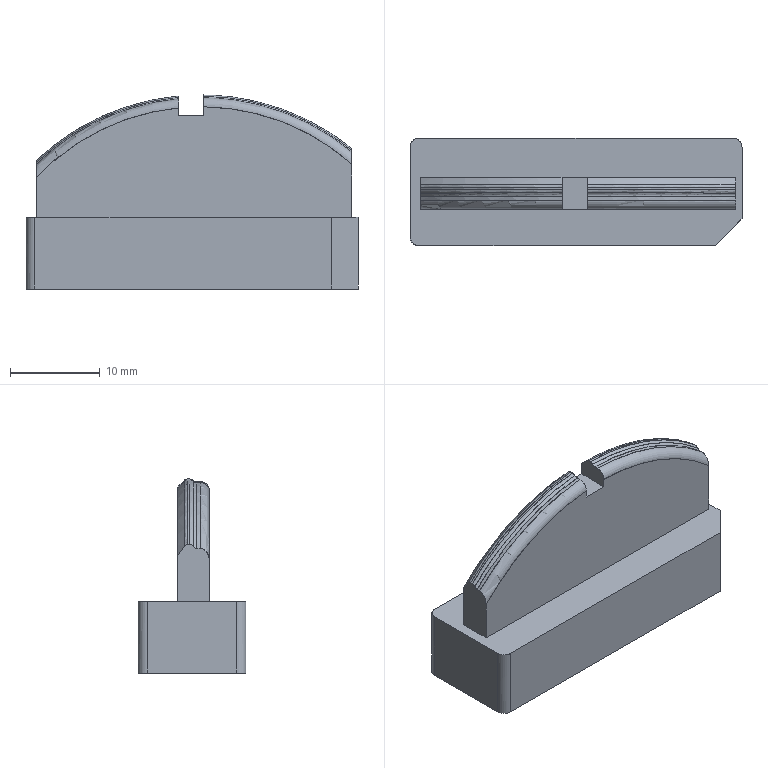NC program | PowerMill | posted with a generic post | part box 37 x 12 x 21.629 mm
Lines 1 to 1018 of 105205:
%
O0001
N104 ( POWERMILL CB  : 2026004.0)
N105 ( POST VER      : 2026.0.0.5161)
N106 ( OPTION FILE   : FANUC)
N107 ( OUTPUT WORKPLANE : WORLD)
N108 (  )
N109 ( TOOL LIST )
N110 (---------------------------------------)
N111 ( NO. | ID        | DIA.| TIP RAD|LENGTH)
N112 (---------------------------------------)
N113 (    1|D10C_1_1_1 |10.0 |  0.0   |77.08 )
N114 (    2|D4C_1_1    | 4.0 |  0.0   | 68.8 )
N115 (   28|D2C_1_1    | 2.0 |  0.0   |57.56 )
N116 (    3|D10_1_1_1  |10.0 |  0.0   | 76.8 )
N117 (    4|R1_1_1     | 2.0 |  1.0   |65.24 )
N118 (   12|D2_1_1     | 2.0 |  0.0   |57.68 )
N119 (    6|R0.5_1_1   | 1.0 |  0.5   | 63.2 )
N120 (   13|TEXT_D4_1_1| 4.0 |  0.3   |68.88 )
N121 (---------------------------------------)
N122 (  )
N123 ( NUMBER OF TOOLPATHS: 12.0 )
N124 ( ESTIMATED PROGRAM DURATION: 0 HOURS 8 MIN 47 SEC)
N125 (  )
N126 G00 G21 G80 G40 G17
N127 G90
N128 G54
N129 G53 Z0.0
N130 (---------------)
N131 ( START TOOLPATH : 精公开粗01-扫面平行-D10C )
N132 (---------------)
N133 ( TOOL NO.    :1 )
N134 ( TOOL TYPE   : ENDMILL)
N135 ( TOOL ID     : D10C_1_1_1)
N136 ( TOOL DIA    : 10.0 LENGTH 77.08)
N137 T1
N138 M6
N139 S8000 M03
N140 G00 G90 X0.0 Y0.0
N141 G43 Z10.2 H1
N142
N143 G05 P10000 R4
N144 X26.28 Y8.78
N145 Z1.129
N146 G01 Z-0.071 F6000.0
N147 X21.28 F10000.0
N148 X-21.28
N149 Y2.9267
N150 X21.28
N151 Y-2.9267
N152 X-21.28
N153 Y-8.78
N154 X21.28
N155 X26.28
N156 G00 Z10.2
N157 G05 P0
N158 (---------------)
N159 ( END TOOLPATH : 精公开粗01-扫面平行-D10C )
N160 (---------------)
N161 ( START TOOLPATH : 精公开粗01-外形偏置-D10C )
N162 (---------------)
N163 G00 X0.242 Y-0.1675 Z9.879
N164 G05 P10000 R4
N165 X-3.7058 Y14.649
N166 Z0.6814
N167 G01 Z-0.5186 F6000.0
N168 Y14.1215 F10000.0
N169 G03 X1.0417 Y9.374 I4.7475 J0.0
N170 G01 X24.573
N171 G02 X25.573 Y8.374 I0.0 J-1.0
N172 G01 Y-8.709
N173 G02 X24.573 Y-9.709 I-1.0 J0.0
N174 G01 X-24.089
N175 G02 X-25.089 Y-8.709 I0.0 J1.0
N176 G01 Y8.374
N177 G02 X-24.089 Y9.374 I1.0 J0.0
N178 G01 X1.0417
N179 X1.2088 Y6.3133
N180 X1.4021 Y6.3238
N181 X2.949 Y6.2597
N182 X3.7224 Y6.2023
N183 X5.3688 Y6.0199
N184 X6.0427 Y5.8933
N185 X6.8161 Y5.6829
N186 X7.5896 Y5.3718
N187 X7.8472 Y5.2465
N188 X8.363 Y4.9346
N189 X8.9527 Y4.4731
N190 X9.6513 Y3.6996
N191 X9.9098 Y3.3388
N192 X10.1534 Y2.9262
N193 X10.4864 Y2.1528
N194 X10.6833 Y1.3714
N195 X10.7117 Y1.0849
N196 X16.2576 Y1.3418
N197 X16.2439 Y1.6377
N198 G02 X17.3399 Y3.2854 I1.6702 J0.0774
N199 G01 X17.6988 Y3.4167
N200 G02 X19.945 Y1.8531 I0.5742 J-1.5703
N201 G01 X19.9612 Y-2.1531
N202 G02 X17.0031 Y-3.5452 I-1.8032 J-0.0073
N203 G01 X16.7549 Y-3.3382
N204 G02 X16.1376 Y-1.8427 I1.1128 J1.3345
N205 G01 X16.2447 Y-0.6921
N206 X16.2894 Y0.0777
N207 X16.2805 Y0.8487
N208 X16.2576 Y1.3418
N209 X10.7117 Y1.0849
N210 X10.7593 Y0.6059
N211 X10.7454 Y-0.1675
N212 X10.6264 Y-0.9409
N213 X10.3838 Y-1.7144
N214 X9.9952 Y-2.4878
N215 X9.4263 Y-3.2612
N216 X9.1364 Y-3.5758
N217 X8.6195 Y-4.0346
N218 X8.363 Y-4.2201
N219 X7.5896 Y-4.654
N220 X6.8161 Y-4.966
N221 X6.1624 Y-5.1488
N222 X6.0948 Y-5.173
N223 X6.0314 Y-5.2067
N224 X5.4336 Y-5.5815
N225 X4.4958 Y-6.0392
N226 X3.7224 Y-6.2668
N227 X3.2355 Y-6.3549
N228 X2.949 Y-6.3912
N229 X1.4021 Y-6.5336
N230 X0.6287 Y-6.4969
N231 X-0.1003 Y-6.3549
N232 X-0.9181 Y-6.0598
N233 X-1.7384 Y-5.5794
N234 X-1.8347 Y-5.536
N235 X-1.9379 Y-5.5137
N236 X-2.465 Y-5.4572
N237 X-4.0118 Y-5.1831
N238 X-4.7853 Y-4.9732
N239 X-5.5587 Y-4.6686
N240 X-6.3321 Y-4.2406
N241 X-6.6232 Y-4.0346
N242 X-7.1056 Y-3.6105
N243 X-7.449 Y-3.2612
N244 X-8.0238 Y-2.4878
N245 X-8.4121 Y-1.7144
N246 X-8.6539 Y-0.9409
N247 X-8.6938 Y-0.6802
N248 X-14.3983 Y-1.0073
N249 X-14.3455 Y-1.9276
N250 G02 X-16.8483 Y-3.977 I-1.9967 J-0.1145
N251 G01 X-17.7043 Y-3.7531
N252 G02 X-19.1982 Y-1.8182 I0.5061 J1.9349
N253 G01 Y1.4832
N254 G02 X-17.6684 Y3.4271 I2.0 J0.0
N255 G01 X-17.0235 Y3.5831
N256 G02 X-14.5566 Y1.7537 I0.4702 J-1.9439
N257 G01 X-14.3983 Y-1.0073
N258 X-8.6938 Y-0.6802
N259 X-8.7721 Y-0.1675
N260 X-8.7879 Y0.6059
N261 X-8.7101 Y1.3794
N262 X-8.5124 Y2.1528
N263 X-8.1804 Y2.9262
N264 X-7.879 Y3.4159
N265 X-7.6758 Y3.6996
N266 X-7.1056 Y4.3308
N267 X-6.3321 Y4.9568
N268 X-5.8498 Y5.2465
N269 X-5.5587 Y5.3869
N270 X-4.7853 Y5.69
N271 X-4.0118 Y5.8981
N272 X-3.3512 Y6.0199
N273 X-1.6916 Y6.2012
N274 X-0.9181 Y6.1653
N275 X-0.4581 Y6.0835
N276 X-0.3402 Y6.0767
N277 X-0.224 Y6.0977
N278 X-0.1447 Y6.122
N279 X0.6287 Y6.2816
N280 X1.2088 Y6.3133
N281 X1.0417 Y9.374
N282 G00 Z3.2838
N283 G01 X-3.7058 Y14.649
N284 G00 Z0.2838
N285 G01 Z-0.9162 F6000.0
N286 Y14.1215 F10000.0
N287 G03 X1.0417 Y9.374 I4.7475 J0.0
N288 G01 X24.573
N289 G02 X25.573 Y8.374 I0.0 J-1.0
N290 G01 Y-0.2376
N291 X19.8931 Y-0.1574
N292 X19.8544 Y-2.8993
N293 G02 X18.8442 Y-3.6348 I-0.7809 J0.011
N294 G01 X18.4957 Y-3.5278
N295 G02 X17.9956 Y-2.7453 I0.2105 J0.6856
N296 G01 X18.2091 Y-1.18
N297 G03 X18.2459 Y1.5707 I-11.186 J1.5254
N298 G01 X18.1442 Y2.5018
N299 G02 X18.6817 Y3.1923 I0.6248 J0.0682
N300 G01 X19.1656 Y3.2602
N301 G02 X19.9318 Y2.5844 I0.0935 J-0.6663
N302 G01 X19.8931 Y-0.1574
N303 X25.573 Y-0.2376
N304 Y-8.709
N305 G02 X24.573 Y-9.709 I-1.0 J0.0
N306 G01 X-24.089
N307 G02 X-25.089 Y-8.709 I0.0 J1.0
N308 G01 Y8.374
N309 G02 X-24.089 Y9.374 I1.0 J0.0
N310 G01 X0.9629
N311 X1.1121 Y6.7052
N312 X1.4021 Y6.7215
N313 X2.949 Y6.6563
N314 X3.7224 Y6.5978
N315 X5.2693 Y6.4317
N316 X7.5896 Y6.0268
N317 X8.363 Y5.8328
N318 X9.1364 Y5.576
N319 X9.804 Y5.2465
N320 X10.6833 Y4.6509
N321 X10.8898 Y4.4731
N322 X11.5828 Y3.6996
N323 X12.0614 Y2.9262
N324 X12.2301 Y2.573
N325 X12.3936 Y2.1528
N326 X12.5912 Y1.3794
N327 X12.6666 Y0.6059
N328 X12.6539 Y-0.1675
N329 X12.5353 Y-0.9409
N330 X12.2911 Y-1.7144
N331 X11.9079 Y-2.4878
N332 X11.3639 Y-3.2612
N333 X10.6833 Y-3.9336
N334 X9.8625 Y-4.4919
N335 X9.8122 Y-4.5311
N336 X9.7673 Y-4.5763
N337 X9.7224 Y-4.6276
N338 X9.1364 Y-5.1826
N339 X8.5886 Y-5.5815
N340 X7.5896 Y-6.1042
N341 X6.956 Y-6.3549
N342 X6.0427 Y-6.6013
N343 X5.2693 Y-6.7489
N344 X4.4958 Y-6.8496
N345 X2.949 Y-6.9772
N346 X1.4021 Y-7.0238
N347 X0.6287 Y-6.9871
N348 X-0.2047 Y-6.8115
N349 X-0.2986 Y-6.8008
N350 X-0.3928 Y-6.808
N351 X-0.9181 Y-6.8986
N352 X-1.6916 Y-6.9275
N353 X-2.465 Y-6.8575
N354 X-3.2384 Y-6.7562
N355 X-4.0118 Y-6.6086
N356 X-4.7853 Y-6.4026
N357 X-5.5587 Y-6.1159
N358 X-6.3321 Y-5.741
N359 X-6.6106 Y-5.5815
N360 X-7.1056 Y-5.2246
N361 X-7.5738 Y-4.8081
N362 X-7.8388 Y-4.5227
N363 X-7.8812 Y-4.4822
N364 X-7.9281 Y-4.4468
N365 X-8.5473 Y-4.0346
N366 X-9.3538 Y-3.2612
N367 X-9.8919 Y-2.4878
N368 X-10.2739 Y-1.7144
N369 X-10.5168 Y-0.9409
N370 X-10.635 Y-0.1675
N371 Y-0.1658
N372 X-16.2712 Y-0.4157
N373 X-16.2674 Y-0.5009
N374 X-16.1342 Y-2.2825
N375 G02 X-17.6603 Y-4.0077 I-1.6027 J-0.1199
N376 G02 X-19.3438 Y-2.4356 I-0.0766 J1.6053
N377 G01 X-19.4362 Y2.0303
N378 G02 X-16.8686 Y3.1779 I1.5262 J0.0316
N379 G01 X-16.7304 Y3.0489
N380 G02 X-16.2734 Y1.9733 I-0.9816 J-1.0519
N381 G01 X-16.2977 Y0.1812
N382 X-16.2712 Y-0.4157
N383 X-10.635 Y-0.1658
N384 X-10.6489 Y0.6059
N385 X-10.573 Y1.3794
N386 X-10.3765 Y2.1528
N387 X-10.1993 Y2.6067
N388 X-10.044 Y2.9262
N389 X-9.569 Y3.6996
N390 X-9.4258 Y3.89
N391 X-8.8796 Y4.4731
N392 X-8.6524 Y4.6669
N393 X-7.879 Y5.1956
N394 X-7.1056 Y5.5891
N395 X-6.3321 Y5.8469
N396 X-5.5587 Y6.0303
N397 X-4.0118 Y6.322
N398 X-2.465 Y6.5244
N399 X-1.6916 Y6.5964
N400 X-0.9181 Y6.5595
N401 X-0.4624 Y6.4781
N402 X-0.3447 Y6.4711
N403 X-0.2286 Y6.492
N404 X-0.1447 Y6.5176
N405 X0.6287 Y6.6782
N406 X1.1121 Y6.7052
N407 X0.9629 Y9.374
N408 X1.0417
N409 G00 Z2.8861
N410 G01 X-3.7058 Y14.649
N411 G00 Z-0.1139
N412 G01 Z-1.3139 F6000.0
N413 Y14.1215 F10000.0
N414 G03 X1.0417 Y9.374 I4.7475 J0.0
N415 G01 X2.9512
N416 X2.949 Y6.8729
N417 X4.4958 Y6.8716
N418 X5.4708 Y6.7933
N419 X7.5896 Y6.414
N420 X9.1364 Y6.0561
N421 X9.9098 Y5.8404
N422 X10.6833 Y5.5459
N423 X11.4567 Y5.1307
N424 X12.2301 Y4.5478
N425 X13.0107 Y3.6996
N426 X13.4819 Y2.9262
N427 X13.777 Y2.2408
N428 X14.0066 Y1.3794
N429 X14.0825 Y0.6059
N430 X14.0678 Y-0.1675
N431 X13.95 Y-0.9409
N432 X13.777 Y-1.5309
N433 X13.3301 Y-2.4878
N434 X13.0035 Y-2.9907
N435 X12.7928 Y-3.2612
N436 X12.2301 Y-3.8366
N437 X12.014 Y-4.0144
N438 X11.9644 Y-4.0612
N439 X11.9216 Y-4.1143
N440 X11.4567 Y-4.6934
N441 X10.6833 Y-5.3869
N442 X9.9098 Y-5.9011
N443 X9.1364 Y-6.2674
N444 X8.363 Y-6.5411
N445 X7.5896 Y-6.7396
N446 X6.8161 Y-6.894
N447 X5.2693 Y-7.0717
N448 X4.2297 Y-7.1283
N449 X1.4021 Y-7.1856
N450 X0.6287 Y-7.1515
N451 X-0.0851 Y-7.0102
N452 X-0.1785 Y-7.0007
N453 X-0.2721 Y-7.0089
N454 X-0.9181 Y-7.1269
N455 X-1.6916 Y-7.1557
N456 X-3.2384 Y-7.0743
N457 X-4.7853 Y-6.9012
N458 X-5.5587 Y-6.7449
N459 X-6.3321 Y-6.5514
N460 X-6.9147 Y-6.3549
N461 X-7.879 Y-5.9193
N462 X-8.6524 Y-5.3943
N463 X-9.334 Y-4.8081
N464 X-9.7128 Y-4.3808
N465 X-9.8966 Y-4.1287
N466 X-9.9372 Y-4.08
N467 X-9.9835 Y-4.0368
N468 X-10.1993 Y-3.8598
N469 X-10.7912 Y-3.2612
N470 X-10.9727 Y-3.0292
N471 X-11.3287 Y-2.4878
N472 X-11.7125 Y-1.7144
N473 X-11.8563 Y-1.2605
N474 X-17.1845 Y-2.3028
N475 X-17.1233 Y-2.6155
N476 G02 X-17.5543 Y-3.7187 I-1.0844 J-0.2122
N477 G01 X-17.7752 Y-3.8806
N478 G02 X-19.6195 Y-2.9372 I-0.6853 J0.9346
N479 G01 X-19.5771 Y2.682
N480 G02 X-18.2738 Y3.5913 I0.974 J-0.0074
N481 G01 X-18.0042 Y3.4944
N482 G02 X-17.3823 Y2.5501 I-0.3185 J-0.8867
N483 G01 X-17.4739 Y1.0567
N484 G03 X-17.2864 Y-1.7817 I11.1884 J-0.6863
N485 G01 X-17.1845 Y-2.3028
N486 X-11.8563 Y-1.2605
N487 X-11.9575 Y-0.9409
N488 X-12.0758 Y-0.1675
N489 X-12.0886 Y0.6059
N490 X-12.0138 Y1.3794
N491 X-11.818 Y2.1528
N492 X-11.4888 Y2.9262
N493 X-11.0087 Y3.6996
N494 X-10.317 Y4.4731
N495 X-9.4258 Y5.1474
N496 X-8.6524 Y5.5581
N497 X-7.879 Y5.8503
N498 X-7.2392 Y6.0199
N499 X-5.5587 Y6.4207
N500 X-4.0118 Y6.7135
N501 X-3.4503 Y6.7933
N502 X-2.465 Y6.8715
N503 X-1.6916 Y6.8743
N504 X-0.9181 Y6.8353
N505 X-0.2241 Y6.6958
N506 X-0.1247 Y6.686
N507 X-0.0253 Y6.6962
N508 X0.6287 Y6.8301
N509 X1.4021 Y6.8743
N510 X2.949 Y6.8729
N511 X2.9512 Y9.374
N512 X24.573
N513 G02 X25.573 Y8.374 I0.0 J-1.0
N514 G01 Y3.3475
N515 X19.947 Y3.1278
N516 G02 X19.3935 Y3.0437 I-0.2815 J-0.011
N517 G01 X19.3286 Y3.2851
N518 G02 X19.5074 Y3.5599 I0.2127 J0.0572
N519 G01 X19.6747 Y3.5859
N520 G02 X19.9376 Y3.3695 I0.0351 J-0.2253
N521 G01 X19.947 Y3.1278
N522 X25.573 Y3.3475
N523 Y-4.504
N524 X20.0275 Y-3.5842
N525 G02 X19.2819 Y-3.7313 I-0.4004 J0.0664
N526 G01 X19.1568 Y-3.5291
N527 G02 X19.3996 Y-2.8514 I0.3915 J0.2421
N528 G02 X20.0061 Y-3.2392 I0.1487 J-0.4356
N529 G01 X20.0307 Y-3.4757
N530 X20.0327 Y-3.5301
N531 X20.0275 Y-3.5842
N532 X25.573 Y-4.504
N533 Y-8.709
N534 G02 X24.573 Y-9.709 I-1.0 J0.0
N535 G01 X-24.089
N536 G02 X-25.089 Y-8.709 I0.0 J1.0
N537 G01 Y8.374
N538 G02 X-24.089 Y9.374 I1.0 J0.0
N539 G01 X1.0417
N540 G00 Z2.4885
N541 G01 X-3.7058 Y14.649
N542 G00 Z-0.5115
N543 G01 Z-1.7115 F6000.0
N544 Y14.1215 F10000.0
N545 G03 X1.0417 Y9.374 I4.7475 J0.0
N546 G01 X20.1246
N547 Y4.2468
N548 G02 X20.471 Y3.9004 I0.0 J-0.3464
N549 G02 X19.7783 I-0.3464 J0.0
N550 G02 X20.1246 Y4.2468 I0.3463 J0.0
N551 G01 Y9.374
N552 X24.573
N553 G02 X25.573 Y8.374 I0.0 J-1.0
N554 G01 Y-8.709
N555 G02 X24.573 Y-9.709 I-1.0 J0.0
N556 G01 X19.968
N557 Y-4.7019
N558 G02 X19.3943 Y-4.1282 I0.0 J0.5737
N559 G02 X20.5417 I0.5737 J0.0
N560 G02 X19.968 Y-4.7019 I-0.5737 J0.0
N561 G01 Y-9.709
N562 X3.3474
N563 X3.3357 Y-7.2005
N564 X1.4021 Y-7.2096
N565 X0.6287 Y-7.1728
N566 X-0.0222 Y-7.0476
N567 X-0.1239 Y-7.0386
N568 X-0.2253 Y-7.0505
N569 X-0.5749 Y-7.1283
N570 X-0.9181 Y-7.1762
N571 X-1.6916 Y-7.2096
N572 X-4.0118 Y-7.1716
N573 X-5.5587 Y-7.0472
N574 X-6.3321 Y-6.9302
N575 X-7.1056 Y-6.7652
N576 X-7.879 Y-6.5567
N577 X-8.4179 Y-6.3549
N578 X-9.4258 Y-5.8455
N579 X-9.8237 Y-5.5815
N580 X-10.1993 Y-5.2774
N581 X-10.7112 Y-4.8081
N582 X-10.9727 Y-4.521
N583 X-11.3345 Y-4.0346
N584 X-11.986 Y-3.2612
N585 X-12.5195 Y-2.4947
N586 X-12.8917 Y-1.7144
N587 X-13.1014 Y-1.0429
N588 X-17.8642 Y-1.9141
N589 X-17.6455 Y-3.11
N590 G02 X-18.081 Y-4.1629 I-1.0335 J-0.189
N591 G01 X-18.3526 Y-4.3509
N592 G02 X-20.1568 Y-3.4137 I-0.6544 J0.9454
N593 G01 X-20.2035 Y3.1186
N594 G02 X-18.942 Y4.0611 I0.9777 J0.007
N595 G01 X-18.5197 Y3.933
N596 G02 X-17.8832 Y2.9673 I-0.2626 J-0.8657
N597 G01 X-18.0438 Y1.5228
N598 G03 X-17.9372 Y-1.5155 I10.3971 J-1.156
N599 G01 X-17.8642 Y-1.9141
N600 X-13.1014 Y-1.0429
N601 X-13.1332 Y-0.9409
N602 X-13.2512 Y-0.1675
N603 X-13.2647 Y0.6059
N604 X-13.1892 Y1.3794
N605 X-12.9928 Y2.1528
N606 X-12.6737 Y2.9262
N607 X-12.5195 Y3.2134
N608 X-12.207 Y3.6996
N609 X-11.7461 Y4.2445
N610 X-11.512 Y4.4731
N611 X-10.9727 Y4.9204
N612 X-10.4886 Y5.2465
N613 X-10.1993 Y5.406
N614 X-9.4258 Y5.7491
N615 X-7.879 Y6.2368
N616 X-7.1056 Y6.4391
N617 X-5.6092 Y6.7933
N618 X-4.7853 Y6.8702
N619 X-1.6916 Y6.8743
N620 X-0.9181 Y6.8353
N621 X-0.2241 Y6.6958
N622 X-0.1247 Y6.686
N623 X-0.0253 Y6.6962
N624 X0.6287 Y6.8302
N625 X1.4021 Y6.8743
N626 X1.6056 Y6.8741
N627 X4.4958 Y6.8715
N628 X4.5054 Y6.8707
N629 X6.8161 Y6.8681
N630 X7.5722 Y6.7933
N631 X9.1364 Y6.4402
N632 X11.4567 Y5.7421
N633 X12.2301 Y5.3918
N634 X12.4926 Y5.2465
N635 X13.0035 Y4.9005
N636 X13.5158 Y4.4731
N637 X13.777 Y4.2142
N638 X14.2068 Y3.6996
N639 X14.6746 Y2.9262
N640 X14.9897 Y2.1528
N641 X15.1863 Y1.3794
N642 X15.2621 Y0.6059
N643 X15.2479 Y-0.1675
N644 X15.1302 Y-0.9409
N645 X14.8877 Y-1.7144
N646 X14.5264 Y-2.4878
N647 X13.9897 Y-3.2612
N648 X13.777 Y-3.4985
N649 X13.0035 Y-4.4877
N650 X12.7181 Y-4.8081
N651 X12.2301 Y-5.2606
N652 X11.8327 Y-5.5815
N653 X11.4567 Y-5.8369
N654 X10.6833 Y-6.2334
N655 X9.9098 Y-6.5422
N656 X9.1364 Y-6.7578
N657 X8.363 Y-6.9272
N658 X7.5896 Y-7.0416
N659 X6.666 Y-7.1283
N660 X5.2693 Y-7.1915
N661 X3.3357 Y-7.2005
N662 X3.3474 Y-9.709
N663 X-24.089
N664 G02 X-25.089 Y-8.709 I0.0 J1.0
N665 G01 Y8.374
N666 G02 X-24.089 Y9.374 I1.0 J0.0
N667 G01 X1.0417
N668 G00 Z2.0909
N669 G01 X-3.7058 Y14.649
N670 G00 Z-0.9091
N671 G01 Z-2.1091 F6000.0
N672 Y14.1215 F10000.0
N673 G03 X1.0417 Y9.374 I4.7475 J0.0
N674 G01 X4.4958
N675 Y6.8743
N676 X7.5896
N677 X8.363 Y6.8676
N678 X9.0988 Y6.7933
N679 X9.9098 Y6.5996
N680 X10.6833 Y6.3701
N681 X12.2301 Y5.853
N682 X13.0035 Y5.5397
N683 X13.777 Y5.1052
N684 X14.5582 Y4.4731
N685 X15.2485 Y3.6996
N686 X15.7158 Y2.9262
N687 X16.0311 Y2.1528
N688 X16.227 Y1.3794
N689 X16.303 Y0.6059
N690 X16.2891 Y-0.1675
N691 X16.1695 Y-0.9409
N692 X15.9299 Y-1.7144
N693 X20.1087 Y-3.384
N694 X15.9299 Y-1.7144
N695 X15.5669 Y-2.4878
N696 X15.3238 Y-2.8727
N697 X14.5504 Y-3.9486
N698 X13.8727 Y-4.8081
N699 X13.0246 Y-5.5815
N700 X12.2301 Y-6.0706
N701 X11.6516 Y-6.3549
N702 X10.6833 Y-6.6946
N703 X9.9098 Y-6.8941
N704 X9.1364 Y-7.0363
N705 X8.287 Y-7.1283
N706 X7.5896 Y-7.1807
N707 X6.8161 Y-7.2024
N708 X1.4021 Y-7.2096
N709 X0.6287 Y-7.1729
N710 X-0.029 Y-7.0463
N711 X-0.0307 Y-7.046
N712 X-0.0324 Y-7.0457
N713 X-0.1291 Y-7.0387
N714 X-0.2253 Y-7.0505
N715 X-0.5749 Y-7.1283
N716 X-0.8162 Y-7.1619
N717 X-0.9181 Y-7.1816
N718 X-1.6916 Y-7.2096
N719 X-4.0118
N720 X-5.5587 Y-7.1812
N721 X-7.1056 Y-7.043
N722 X-7.879 Y-6.899
N723 X-8.6524 Y-6.7043
N724 X-9.4258 Y-6.4531
N725 X-10.1993 Y-6.0838
N726 X-10.9727 Y-5.6101
N727 X-11.869 Y-4.8081
N728 X-12.5195 Y-3.9893
N729 X-13.293 Y-2.9152
N730 X-13.5663 Y-2.4878
N731 X-13.9257 Y-1.7144
N732 X-14.1649 Y-0.9409
N733 X-14.2829 Y-0.1675
N734 X-14.2968 Y0.6059
N735 X-14.221 Y1.3794
N736 X-14.0664 Y2.0181
N737 X-13.7122 Y2.9262
N738 X-13.293 Y3.6326
N739 X-12.5564 Y4.4731
N740 X-11.7461 Y5.1219
N741 X-10.9727 Y5.5484
N742 X-10.1993 Y5.8674
N743 X-7.879 Y6.6171
N744 X-7.1282 Y6.7933
N745 X-6.3321 Y6.8707
N746 X-1.6916 Y6.8743
N747 X-0.9181 Y6.8353
N748 X-0.2242 Y6.6958
N749 X-0.1247 Y6.686
N750 X-0.0252 Y6.6962
N751 X0.6287 Y6.8302
N752 X1.4021 Y6.8743
N753 X4.4958
N754 Y9.374
N755 X24.573
N756 G02 X25.573 Y8.374 I0.0 J-1.0
N757 G01 Y4.2565
N758 X21.073
N759 X25.573
N760 Y-8.709
N761 G02 X24.573 Y-9.709 I-1.0 J0.0
N762 G01 X-24.089
N763 G02 X-25.089 Y-8.709 I0.0 J1.0
N764 G01 Y-0.1675
N765 X-20.589
N766 Y4.374
N767 G02 X-20.089 Y4.874 I0.5 J0.0
N768 G01 X-18.5143
N769 G02 X-18.0485 Y4.1923 I0.0 J-0.5
N770 G01 X-18.2587 Y3.6534
N771 X-18.3591 Y3.3681
N772 X-18.4401 Y3.0767
N773 X-18.5947 Y2.438
N774 X-18.658 Y2.1299
N775 X-18.6995 Y1.8182
N776 X-18.7753 Y1.0448
N777 X-18.7932 Y0.7852
N778 X-18.7961 Y0.5251
N779 X-18.7822 Y-0.2484
N780 X-18.7668 Y-0.548
N781 X-18.7314 Y-0.8459
N782 X-18.6135 Y-1.6193
N783 X-18.5509 Y-1.9477
N784 X-18.464 Y-2.2706
N785 X-18.2248 Y-3.044
N786 X-18.1253 Y-3.331
N787 X-18.0067 Y-3.6106
N788 X-17.6473 Y-4.384
N789 X-17.6229 Y-4.4356
N790 X-17.5979 Y-4.4869
N791 G02 X-18.0459 Y-5.209 I-0.448 J-0.2221
N792 G01 X-20.089
N793 G02 X-20.589 Y-4.709 I0.0 J0.5
N794 G01 Y-0.1675
N795 X-25.089
N796 Y8.374
N797 G02 X-24.089 Y9.374 I1.0 J0.0
N798 G01 X1.0417
N799 G00 Z1.6933
N800 G01 X-3.7058 Y14.649
N801 G00 Z-1.3067
N802 G01 Z-2.5067 F6000.0
N803 Y14.1215 F10000.0
N804 G03 X1.0417 Y9.374 I4.7475 J0.0
N805 G01 X24.573
N806 G02 X25.573 Y8.374 I0.0 J-1.0
N807 G01 Y-8.709
N808 G02 X24.573 Y-9.709 I-1.0 J0.0
N809 G01 X-24.089
N810 G02 X-25.089 Y-8.709 I0.0 J1.0
N811 G01 Y-3.0579
N812 X-20.589
N813 X-25.089
N814 Y3.2919
N815 X-20.589
N816 X-25.089
N817 Y8.374
N818 G02 X-24.089 Y9.374 I1.0 J0.0
N819 G01 X1.0154
N820 Y6.8743
N821 X9.1364
N822 X9.9098 Y6.8507
N823 X10.6833 Y6.7267
N824 X11.4567 Y6.4927
N825 X12.7925 Y6.0199
N826 X13.777 Y5.6262
N827 X14.5 Y5.2465
N828 X15.3238 Y4.6381
N829 X15.5016 Y4.4731
N830 X16.0972 Y3.8111
N831 X16.6483 Y2.9262
N832 X16.9602 Y2.1528
N833 X17.1553 Y1.3794
N834 X17.2315 Y0.6059
N835 X17.2164 Y-0.1675
N836 X17.1004 Y-0.9409
N837 X16.8605 Y-1.7144
N838 X16.5012 Y-2.4878
N839 X15.9657 Y-3.2612
N840 X15.956 Y-3.2778
N841 X15.5138 Y-4.0346
N842 X15.3238 Y-4.3002
N843 X14.8997 Y-4.8081
N844 X14.5504 Y-5.1656
N845 X14.0573 Y-5.5815
N846 X13.777 Y-5.7749
N847 X13.0035 Y-6.2199
N848 X12.2301 Y-6.5473
N849 X11.4567 Y-6.803
N850 X10.6833 Y-6.9773
N851 X9.5997 Y-7.1283
N852 X9.1364 Y-7.1727
N853 X8.363 Y-7.2014
N854 X6.8178 Y-7.2023
N855 X6.8161
N856 X1.4021 Y-7.2095
N857 X1.3175 Y-7.2055
N858 X-1.6288 Y-7.2073
N859 X-1.6916 Y-7.2095
N860 X-4.0118
N861 X-4.0574 Y-7.2087
N862 X-5.5587 Y-7.2096
N863 X-7.1056 Y-7.1741
N864 X-7.6032 Y-7.1283
N865 X-8.6524 Y-6.9835
N866 X-9.4258 Y-6.8106
N867 X-10.1993 Y-6.5601
N868 X-10.9727 Y-6.2397
N869 X-11.7461 Y-5.7903
N870 X-12.0505 Y-5.5815
N871 X-12.5195 Y-5.1886
N872 X-12.8876 Y-4.8081
N873 X-13.293 Y-4.3319
N874 X-13.5033 Y-4.0346
N875 X-13.9596 Y-3.2612
N876 X-14.4932 Y-2.4878
N877 X-14.8398 Y-1.7665
N878 X-15.1022 Y-0.9409
N879 X-15.2203 Y-0.1675
N880 X-15.2343 Y0.6059
N881 X-15.1584 Y1.3794
N882 X-14.963 Y2.1528
N883 X-14.6419 Y2.9262
N884 X-14.1756 Y3.6996
N885 X-13.4908 Y4.4731
N886 X-13.293 Y4.6569
N887 X-12.4928 Y5.2465
N888 X-11.7461 Y5.6415
N889 X-9.4258 Y6.5099
N890 X-8.6524 Y6.7337
N891 X-7.879 Y6.8533
N892 X-7.1056 Y6.8743
N893 X1.0154
N894 Y9.374
N895 X1.0417
N896 G00 Z1.2957
N897 G01 X-3.7058 Y14.649
N898 G00 Z-1.7043
N899 G01 Z-2.9043 F6000.0
N900 Y14.1215 F10000.0
N901 G03 X1.0417 Y9.374 I4.7475 J0.0
N902 G01 X24.573
N903 G02 X25.573 Y8.374 I0.0 J-1.0
N904 G01 Y-8.709
N905 G02 X24.573 Y-9.709 I-1.0 J0.0
N906 G01 X-24.089
N907 G02 X-25.089 Y-8.709 I0.0 J1.0
N908 G01 Y-4.1361
N909 X-20.589
N910 X-25.089
N911 Y8.374
N912 G02 X-24.089 Y9.374 I1.0 J0.0
N913 G01 X1.0154
N914 Y6.8743
N915 X9.9098 Y6.8744
N916 X10.6833 Y6.8691
N917 X11.4072 Y6.7933
N918 X12.2301 Y6.587
N919 X13.0035 Y6.3027
N920 X14.5504 Y5.6697
N921 X15.3483 Y5.2465
N922 X16.0972 Y4.7022
N923 X16.3483 Y4.4731
N924 X16.8707 Y3.9038
N925 X17.0273 Y3.6996
N926 X17.4935 Y2.9262
N927 X17.6441 Y2.591
N928 X17.8011 Y2.1528
N929 X17.9948 Y1.3794
N930 X18.0726 Y0.6059
N931 X18.0583 Y-0.1675
N932 X17.9395 Y-0.9409
N933 X17.7053 Y-1.7144
N934 X17.3473 Y-2.4878
N935 X16.8707 Y-3.1895
N936 X16.8586 Y-3.2118
N937 X16.4142 Y-4.0346
N938 X16.0972 Y-4.4658
N939 X15.8052 Y-4.8081
N940 X15.3238 Y-5.2926
N941 X14.967 Y-5.5815
N942 X14.5504 Y-5.8621
N943 X13.777 Y-6.3054
N944 X13.0035 Y-6.6269
N945 X12.2301 Y-6.8614
N946 X11.4567 Y-7.0309
N947 X10.7224 Y-7.1283
N948 X9.9098 Y-7.1894
N949 X9.1364 Y-7.2096
N950 X-7.1056
N951 X-7.879 Y-7.19
N952 X-8.6524 Y-7.1356
N953 X-9.4258 Y-7.0379
N954 X-10.1993 Y-6.8655
N955 X-10.9727 Y-6.6361
N956 X-11.6753 Y-6.3549
N957 X-12.5195 Y-5.886
N958 X-12.979 Y-5.5815
N959 X-13.293 Y-5.328
N960 X-13.8156 Y-4.8081
N961 X-14.4162 Y-4.0346
N962 X-14.8398 Y-3.2544
N963 X-15.3432 Y-2.4878
N964 X-15.6997 Y-1.7144
N965 X-15.9331 Y-0.9409
N966 X-16.0483 Y-0.1675
N967 X-16.0647 Y0.6059
N968 X-15.9865 Y1.3794
N969 X-15.7967 Y2.1528
N970 X-15.4902 Y2.9262
N971 X-15.0236 Y3.6996
N972 X-14.8398 Y3.935
N973 X-14.3523 Y4.4731
N974 X-14.0664 Y4.7343
N975 X-13.3533 Y5.2465
N976 X-12.5195 Y5.6828
N977 X-10.1993 Y6.6012
N978 X-9.4258 Y6.7916
N979 X-8.6524 Y6.8703
N980 X-7.879 Y6.8743
N981 X1.0154
N982 Y9.374
N983 X1.0417
N984 G00 Z0.8981
N985 G01 X-3.7058 Y14.649
N986 G00 Z-2.1019
N987 G01 Z-3.3019 F6000.0
N988 Y14.1215 F10000.0
N989 G03 X1.0417 Y9.374 I4.7475 J0.0
N990 G01 X24.573
N991 G02 X25.573 Y8.374 I0.0 J-1.0
N992 G01 Y-8.709
N993 G02 X24.573 Y-9.709 I-1.0 J0.0
N994 G01 X1.0154
N995 Y-7.2096
N996 X-7.879
N997 X-8.6524 Y-7.2016
N998 X-9.4258 Y-7.1608
N999 X-10.1993 Y-7.0604
N1000 X-10.9727 Y-6.904
N1001 X-11.7461 Y-6.6811
N1002 X-12.5195 Y-6.3599
N1003 X-13.293 Y-5.9353
N1004 X-13.8018 Y-5.5815
N1005 X-14.0664 Y-5.3686
N1006 X-14.6379 Y-4.8081
N1007 X-15.2331 Y-4.0346
N1008 X-15.6132 Y-3.3513
N1009 X-16.1177 Y-2.4878
N1010 X-16.3867 Y-1.9363
N1011 X-16.7108 Y-0.9409
N1012 X-16.8284 Y-0.1675
N1013 X-16.8425 Y0.6059
N1014 X-16.7665 Y1.3794
N1015 X-16.5718 Y2.1528
N1016 X-16.2652 Y2.9262
N1017 X-15.7986 Y3.6996
N1018 X-15.6132 Y3.9374
N1019 X-15.1274 Y4.4731
N1020 X-14.8398 Y4.7363
N1021 X-14.1308 Y5.2465
N1022 X-13.293 Y5.6953
N1023 X-11.7461 Y6.363
N1024 X-10.9727 Y6.6517
N1025 X-10.3596 Y6.7933
N1026 X-9.4258 Y6.8744
N1027 X-2.2855 Y6.8743
N1028 X9.9098
N1029 X9.9239 Y6.8742
N1030 X11.4567
N1031 X12.2301 Y6.8136
N1032 X13.0035 Y6.6455
N1033 X13.777 Y6.3507
N1034 X15.3238 Y5.6733
N1035 X16.0972 Y5.263
N1036 X16.8707 Y4.7034
N1037 X17.1221 Y4.4731
N1038 X17.7911 Y3.6996
N1039 X18.2576 Y2.9262
N1040 X18.5641 Y2.1528
N1041 X18.7615 Y1.3794
N1042 X18.8371 Y0.6059
N1043 X18.8234 Y-0.1675
N1044 X18.7053 Y-0.9409
N1045 X18.4694 Y-1.7144
N1046 X18.1106 Y-2.4878
N1047 X17.6441 Y-3.2668
N1048 X17.639 Y-3.2763
N1049 X17.228 Y-4.0346
N1050 X16.6359 Y-4.8081
N1051 X16.0972 Y-5.3403
N1052 X15.3238 Y-5.9166
N1053 X14.5504 Y-6.347
N1054 X13.777 Y-6.6742
N1055 X13.0035 Y-6.8934
N1056 X12.2301 Y-7.0553
N1057 X11.716 Y-7.1283
N1058 X10.6833 Y-7.1999
N1059 X9.9098 Y-7.2096
N1060 X1.0154
N1061 Y-9.709
N1062 X-24.089
N1063 G02 X-25.089 Y-8.709 I0.0 J1.0
N1064 G01 Y8.374
N1065 G02 X-24.089 Y9.374 I1.0 J0.0
N1066 G01 X1.0417
N1067 G00 Z0.5005
N1068 G01 X-3.7058 Y14.649
N1069 G00 Z-2.4995
N1070 G01 Z-3.6995 F6000.0
N1071 Y14.1215 F10000.0
N1072 G03 X1.0417 Y9.374 I4.7475 J0.0
N1073 G01 X24.573
N1074 G02 X25.573 Y8.374 I0.0 J-1.0
N1075 G01 Y-8.709
N1076 G02 X24.573 Y-9.709 I-1.0 J0.0
N1077 G01 X-24.089
N1078 G02 X-25.089 Y-8.709 I0.0 J1.0
N1079 G01 Y8.374
N1080 G02 X-24.089 Y9.374 I1.0 J0.0
N1081 G01 X1.0154
N1082 Y6.8744
N1083 X12.2301
N1084 X13.0035 Y6.8258
N1085 X13.777 Y6.6655
N1086 X14.5504 Y6.3844
N1087 X16.0972 Y5.6613
N1088 X16.8631 Y5.2465
N1089 X17.6441 Y4.6635
N1090 X17.8461 Y4.4731
N1091 X18.4175 Y3.8171
N1092 X18.9722 Y2.9262
N1093 X19.2802 Y2.1528
N1094 X19.4679 Y1.3794
N1095 X19.5436 Y0.6059
N1096 X19.5298 Y-0.1675
N1097 X19.4121 Y-0.9409
N1098 X19.1909 Y-1.697
N1099 X18.8274 Y-2.4878
N1100 X17.9871 Y-4.0346
N1101 X17.4092 Y-4.8081
N1102 X16.8707 Y-5.341
N1103 X16.0972 Y-5.9327
N1104 X15.3238 Y-6.3577
N1105 X14.5504 Y-6.6823
N1106 X13.777 Y-6.9101
N1107 X12.6165 Y-7.1283
N1108 X11.4567 Y-7.2062
N1109 X10.0547 Y-7.2077
N1110 X9.9098 Y-7.2095
N1111 X8.4153
N1112 X8.363 Y-7.2096
N1113 X7.9281 Y-7.2095
N1114 X-7.879
N1115 X-8.0859 Y-7.2074